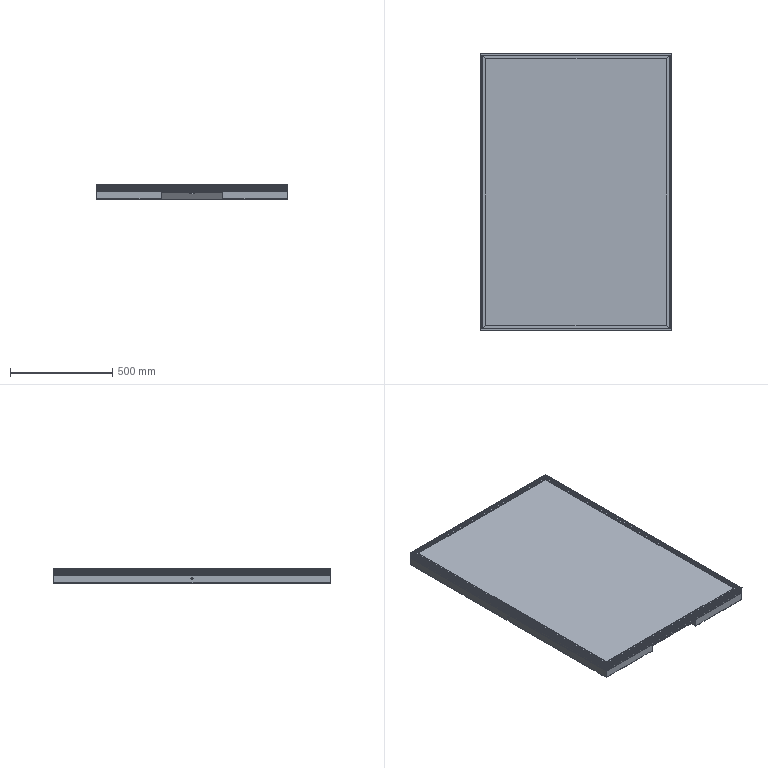Part | SolidWorks | 9 solids | 894 faces | box 940 x 1360 x 70 mm | volume 22273883 mm3 | plane 590 | cylinder 272 | spline 32 | commonest cylinder face diameters 7 x100 0.4 x67 2.4 x41 11 x28 2 x16 10 x12